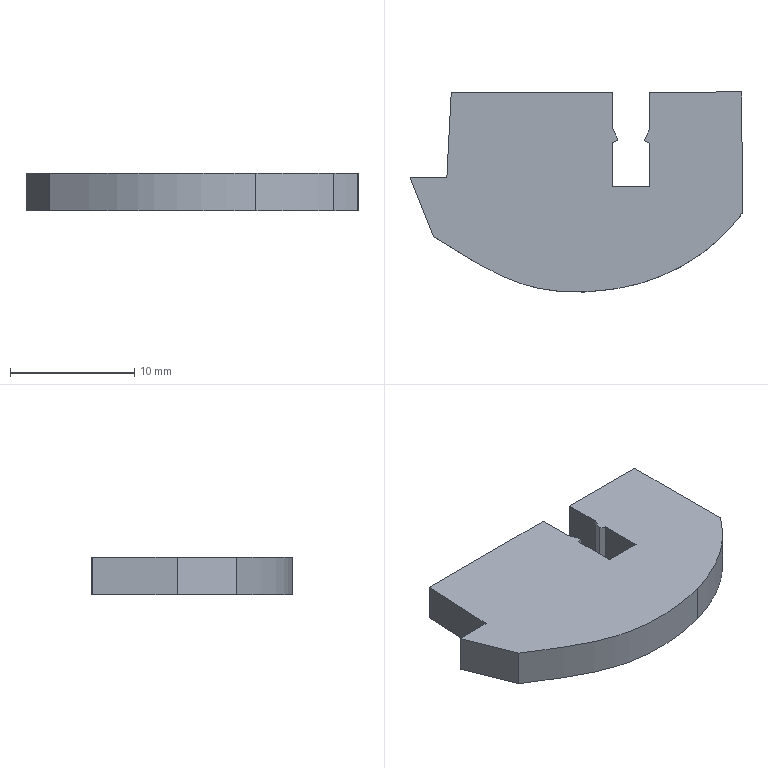Part | SolidWorks | features BaseBody 1 | 1 solid | 22 faces | box 26.677 x 16.089 x 3 mm | volume 988.858 mm3 | plane 18 | spline 4
STEP:
#1=CARTESIAN_POINT('',(-14.822,-11.074,-1.5));
#2=VERTEX_POINT('',#1);
#3=CARTESIAN_POINT('',(-16.703,-6.31,-1.5));
#4=VERTEX_POINT('',#3);
#5=CARTESIAN_POINT('',(-16.606,-6.554,-1.5));
#6=DIRECTION('',(-0.3671,0.9302,0.));
#7=VECTOR('',#6,1000.);
#8=LINE('',#5,#7);
#9=EDGE_CURVE('',#2,#4,#8,.T.);
#10=ORIENTED_EDGE('',*,*,#9,.T.);
#11=CARTESIAN_POINT('',(-13.741,-6.302,-1.5));
#12=VERTEX_POINT('',#11);
#13=CARTESIAN_POINT('',(0.01595,-6.267,-1.5));
#14=DIRECTION('',(1.,0.002545,0.));
#15=VECTOR('',#14,1000.);
#16=LINE('',#13,#15);
#17=EDGE_CURVE('',#4,#12,#16,.T.);
#18=ORIENTED_EDGE('',*,*,#17,.T.);
#19=CARTESIAN_POINT('',(-13.391,0.4792,-1.5));
#20=VERTEX_POINT('',#19);
#21=CARTESIAN_POINT('',(-13.381,0.6903,-1.5));
#22=DIRECTION('',(0.05152,0.9987,0.));
#23=VECTOR('',#22,1000.);
#24=LINE('',#21,#23);
#25=EDGE_CURVE('',#12,#20,#24,.T.);
#26=ORIENTED_EDGE('',*,*,#25,.T.);
#27=CARTESIAN_POINT('',(-0.4409,0.5122,-1.5));
#28=VERTEX_POINT('',#27);
#29=CARTESIAN_POINT('',(-0.001307,0.5133,-1.5));
#30=DIRECTION('',(1.,0.002545,0.));
#31=VECTOR('',#30,1000.);
#32=LINE('',#29,#31);
#33=EDGE_CURVE('',#20,#28,#32,.T.);
#34=ORIENTED_EDGE('',*,*,#33,.T.);
#35=CARTESIAN_POINT('',(-0.4409,-2.331,-1.5));
#36=VERTEX_POINT('',#35);
#37=CARTESIAN_POINT('',(-0.4409,0.,-1.5));
#38=DIRECTION('',(0.,1.,0.));
#39=VECTOR('',#38,1000.);
#40=LINE('',#37,#39);
#41=EDGE_CURVE('',#36,#28,#40,.T.);
#42=ORIENTED_EDGE('',*,*,#41,.F.);
#43=CARTESIAN_POINT('',(0.008047,-3.34,-1.5));
#44=VERTEX_POINT('',#43);
#45=CARTESIAN_POINT('',(-1.234,-0.5495,-1.5));
#46=DIRECTION('',(-0.4068,0.9135,0.));
#47=VECTOR('',#46,1000.);
#48=LINE('',#45,#47);
#49=EDGE_CURVE('',#44,#36,#48,.T.);
#50=ORIENTED_EDGE('',*,*,#49,.F.);
#51=CARTESIAN_POINT('',(-0.4409,-3.537,-1.5));
#52=VERTEX_POINT('',#51);
#53=CARTESIAN_POINT('',(1.232,-2.801,-1.5));
#54=DIRECTION('',(0.9154,0.4025,0.));
#55=VECTOR('',#54,1000.);
#56=LINE('',#53,#55);
#57=EDGE_CURVE('',#52,#44,#56,.T.);
#58=ORIENTED_EDGE('',*,*,#57,.F.);
#59=CARTESIAN_POINT('',(-0.4409,-7.047,-1.5));
#60=VERTEX_POINT('',#59);
#61=CARTESIAN_POINT('',(-0.4409,0.,-1.5));
#62=DIRECTION('',(0.,1.,0.));
#63=VECTOR('',#62,1000.);
#64=LINE('',#61,#63);
#65=EDGE_CURVE('',#60,#52,#64,.T.);
#66=ORIENTED_EDGE('',*,*,#65,.F.);
#67=CARTESIAN_POINT('',(2.555,-7.047,-1.5));
#68=VERTEX_POINT('',#67);
#69=CARTESIAN_POINT('',(0.,-7.047,-1.5));
#70=DIRECTION('',(-1.,0.,0.));
#71=VECTOR('',#70,1000.);
#72=LINE('',#69,#71);
#73=EDGE_CURVE('',#68,#60,#72,.T.);
#74=ORIENTED_EDGE('',*,*,#73,.F.);
#75=CARTESIAN_POINT('',(2.555,-3.572,-1.5));
#76=VERTEX_POINT('',#75);
#77=CARTESIAN_POINT('',(2.555,0.,-1.5));
#78=DIRECTION('',(0.,-1.,0.));
#79=VECTOR('',#78,1000.);
#80=LINE('',#77,#79);
#81=EDGE_CURVE('',#76,#68,#80,.T.);
#82=ORIENTED_EDGE('',*,*,#81,.F.);
#83=CARTESIAN_POINT('',(2.106,-3.373,-1.5));
#84=VERTEX_POINT('',#83);
#85=CARTESIAN_POINT('',(-0.904,-2.036,-1.5));
#86=DIRECTION('',(0.914,-0.4058,0.));
#87=VECTOR('',#86,1000.);
#88=LINE('',#85,#87);
#89=EDGE_CURVE('',#84,#76,#88,.T.);
#90=ORIENTED_EDGE('',*,*,#89,.F.);
#91=CARTESIAN_POINT('',(2.555,-2.414,-1.5));
#92=VERTEX_POINT('',#91);
#93=CARTESIAN_POINT('',(3.023,-1.416,-1.5));
#94=DIRECTION('',(-0.4242,-0.9056,0.));
#95=VECTOR('',#94,1000.);
#96=LINE('',#93,#95);
#97=EDGE_CURVE('',#92,#84,#96,.T.);
#98=ORIENTED_EDGE('',*,*,#97,.F.);
#99=CARTESIAN_POINT('',(2.555,0.5198,-1.5));
#100=VERTEX_POINT('',#99);
#101=CARTESIAN_POINT('',(2.555,0.,-1.5));
#102=DIRECTION('',(0.,-1.,0.));
#103=VECTOR('',#102,1000.);
#104=LINE('',#101,#103);
#105=EDGE_CURVE('',#100,#92,#104,.T.);
#106=ORIENTED_EDGE('',*,*,#105,.F.);
#107=CARTESIAN_POINT('',(9.963,0.5387,-1.5));
#108=VERTEX_POINT('',#107);
#109=CARTESIAN_POINT('',(-0.001307,0.5133,-1.5));
#110=DIRECTION('',(1.,0.002545,0.));
#111=VECTOR('',#110,1000.);
#112=LINE('',#109,#111);
#113=EDGE_CURVE('',#100,#108,#112,.T.);
#114=ORIENTED_EDGE('',*,*,#113,.T.);
#115=CARTESIAN_POINT('',(9.974,-3.538,-1.5));
#116=VERTEX_POINT('',#115);
#117=CARTESIAN_POINT('',(9.965,0.02536,-1.5));
#118=DIRECTION('',(0.002545,-1.,0.));
#119=VECTOR('',#118,1000.);
#120=LINE('',#117,#119);
#121=EDGE_CURVE('',#108,#116,#120,.T.);
#122=ORIENTED_EDGE('',*,*,#121,.T.);
#123=CARTESIAN_POINT('',(9.974,-9.237,-1.5));
#124=VERTEX_POINT('',#123);
#125=CARTESIAN_POINT('',(9.974,0.,-1.5));
#126=DIRECTION('',(0.,-1.,0.));
#127=VECTOR('',#126,1000.);
#128=LINE('',#125,#127);
#129=EDGE_CURVE('',#116,#124,#128,.T.);
#130=ORIENTED_EDGE('',*,*,#129,.T.);
#131=CARTESIAN_POINT('',(9.954,-9.263,-1.5));
#132=VERTEX_POINT('',#131);
#133=CARTESIAN_POINT('',(9.974,-9.237,-1.5));
#134=CARTESIAN_POINT('',(9.967,-9.246,-1.5));
#135=CARTESIAN_POINT('',(9.961,-9.255,-1.5));
#136=CARTESIAN_POINT('',(9.954,-9.263,-1.5));
#137=B_SPLINE_CURVE_WITH_KNOTS('',3,(#133,#134,#135,#136),.UNSPECIFIED.,.F.,.F.,(4,4),(0.5,0.5003),.UNSPECIFIED.);
#138=EDGE_CURVE('',#124,#132,#137,.T.);
#139=ORIENTED_EDGE('',*,*,#138,.T.);
#140=CARTESIAN_POINT('',(8.037,-11.399,-1.5));
#141=VERTEX_POINT('',#140);
#142=CARTESIAN_POINT('',(8.037,-11.399,-1.5));
#143=CARTESIAN_POINT('',(8.294,-11.148,-1.5));
#144=CARTESIAN_POINT('',(8.961,-10.455,-1.5));
#145=CARTESIAN_POINT('',(9.572,-9.722,-1.5));
#146=CARTESIAN_POINT('',(9.954,-9.263,-1.5));
#147=B_SPLINE_CURVE_WITH_KNOTS('',3,(#142,#143,#144,#145,#146),.UNSPECIFIED.,.F.,.F.,(4,1,4),(0.895,0.9336,0.9981),.UNSPECIFIED.);
#148=EDGE_CURVE('',#141,#132,#147,.T.);
#149=ORIENTED_EDGE('',*,*,#148,.F.);
#150=CARTESIAN_POINT('',(1.771,-14.856,-1.5));
#151=VERTEX_POINT('',#150);
#152=CARTESIAN_POINT('',(8.037,-11.399,-1.5));
#153=CARTESIAN_POINT('',(6.42,-12.884,-1.5));
#154=CARTESIAN_POINT('',(4.367,-14.099,-1.5));
#155=CARTESIAN_POINT('',(1.771,-14.856,-1.5));
#156=B_SPLINE_CURVE_WITH_KNOTS('',3,(#152,#153,#154,#155),.UNSPECIFIED.,.F.,.F.,(4,4),(0.5252,0.5809),.UNSPECIFIED.);
#157=EDGE_CURVE('',#141,#151,#156,.T.);
#158=ORIENTED_EDGE('',*,*,#157,.T.);
#159=CARTESIAN_POINT('',(-14.822,-11.074,-1.5));
#160=CARTESIAN_POINT('',(-13.537,-11.899,-1.5));
#161=CARTESIAN_POINT('',(-11.104,-13.46,-1.5));
#162=CARTESIAN_POINT('',(-7.073,-15.339,-1.5));
#163=CARTESIAN_POINT('',(-2.98,-15.702,-1.5));
#164=CARTESIAN_POINT('',(-0.01753,-15.28,-1.5));
#165=CARTESIAN_POINT('',(1.443,-14.941,-1.5));
#166=CARTESIAN_POINT('',(1.771,-14.856,-1.5));
#167=B_SPLINE_CURVE_WITH_KNOTS('',3,(#159,#160,#161,#162,#163,#164,#165,#166),.UNSPECIFIED.,.F.,.F.,(4,1,1,1,1,4),(0.,0.1649,0.3121,0.4748,0.5989,0.6352),.UNSPECIFIED.);
#168=EDGE_CURVE('',#2,#151,#167,.T.);
#169=ORIENTED_EDGE('',*,*,#168,.F.);
#170=EDGE_LOOP('',(#10,#18,#26,#34,#42,#50,#58,#66,#74,#82,#90,#98,#106,#114,#122,#130,#139,#149,#158,#169));
#171=FACE_OUTER_BOUND('',#170,.T.);
#172=CARTESIAN_POINT('',(0.,0.,-1.5));
#173=DIRECTION('',(0.,0.,1.));
#174=DIRECTION('',(1.,0.,0.));
#175=AXIS2_PLACEMENT_3D('',#172,#173,#174);
#176=PLANE('',#175);
#177=ADVANCED_FACE('',(#171),#176,.F.);
#178=CARTESIAN_POINT('',(-14.822,-11.074,1.5));
#179=VERTEX_POINT('',#178);
#180=CARTESIAN_POINT('',(-16.703,-6.31,1.5));
#181=VERTEX_POINT('',#180);
#182=CARTESIAN_POINT('',(-16.606,-6.554,1.5));
#183=DIRECTION('',(-0.3671,0.9302,0.));
#184=VECTOR('',#183,1000.);
#185=LINE('',#182,#184);
#186=EDGE_CURVE('',#179,#181,#185,.T.);
#187=ORIENTED_EDGE('',*,*,#186,.F.);
#188=CARTESIAN_POINT('',(1.771,-14.856,1.5));
#189=VERTEX_POINT('',#188);
#190=CARTESIAN_POINT('',(-14.822,-11.074,1.5));
#191=CARTESIAN_POINT('',(-13.537,-11.899,1.5));
#192=CARTESIAN_POINT('',(-11.104,-13.46,1.5));
#193=CARTESIAN_POINT('',(-7.073,-15.339,1.5));
#194=CARTESIAN_POINT('',(-2.98,-15.702,1.5));
#195=CARTESIAN_POINT('',(-0.01753,-15.28,1.5));
#196=CARTESIAN_POINT('',(1.443,-14.941,1.5));
#197=CARTESIAN_POINT('',(1.771,-14.856,1.5));
#198=B_SPLINE_CURVE_WITH_KNOTS('',3,(#190,#191,#192,#193,#194,#195,#196,#197),.UNSPECIFIED.,.F.,.F.,(4,1,1,1,1,4),(0.,0.1649,0.3121,0.4748,0.5989,0.6352),.UNSPECIFIED.);
#199=EDGE_CURVE('',#179,#189,#198,.T.);
#200=ORIENTED_EDGE('',*,*,#199,.T.);
#201=CARTESIAN_POINT('',(8.037,-11.399,1.5));
#202=VERTEX_POINT('',#201);
#203=CARTESIAN_POINT('',(8.037,-11.399,1.5));
#204=CARTESIAN_POINT('',(6.42,-12.884,1.5));
#205=CARTESIAN_POINT('',(4.367,-14.099,1.5));
#206=CARTESIAN_POINT('',(1.771,-14.856,1.5));
#207=B_SPLINE_CURVE_WITH_KNOTS('',3,(#203,#204,#205,#206),.UNSPECIFIED.,.F.,.F.,(4,4),(0.5252,0.5809),.UNSPECIFIED.);
#208=EDGE_CURVE('',#202,#189,#207,.T.);
#209=ORIENTED_EDGE('',*,*,#208,.F.);
#210=CARTESIAN_POINT('',(9.954,-9.263,1.5));
#211=VERTEX_POINT('',#210);
#212=CARTESIAN_POINT('',(8.037,-11.399,1.5));
#213=CARTESIAN_POINT('',(8.294,-11.148,1.5));
#214=CARTESIAN_POINT('',(8.961,-10.455,1.5));
#215=CARTESIAN_POINT('',(9.572,-9.722,1.5));
#216=CARTESIAN_POINT('',(9.954,-9.263,1.5));
#217=B_SPLINE_CURVE_WITH_KNOTS('',3,(#212,#213,#214,#215,#216),.UNSPECIFIED.,.F.,.F.,(4,1,4),(0.895,0.9336,0.9981),.UNSPECIFIED.);
#218=EDGE_CURVE('',#202,#211,#217,.T.);
#219=ORIENTED_EDGE('',*,*,#218,.T.);
#220=CARTESIAN_POINT('',(9.974,-9.237,1.5));
#221=VERTEX_POINT('',#220);
#222=CARTESIAN_POINT('',(9.974,-9.237,1.5));
#223=CARTESIAN_POINT('',(9.967,-9.246,1.5));
#224=CARTESIAN_POINT('',(9.961,-9.255,1.5));
#225=CARTESIAN_POINT('',(9.954,-9.263,1.5));
#226=B_SPLINE_CURVE_WITH_KNOTS('',3,(#222,#223,#224,#225),.UNSPECIFIED.,.F.,.F.,(4,4),(0.5,0.5003),.UNSPECIFIED.);
#227=EDGE_CURVE('',#221,#211,#226,.T.);
#228=ORIENTED_EDGE('',*,*,#227,.F.);
#229=CARTESIAN_POINT('',(9.974,-3.538,1.5));
#230=VERTEX_POINT('',#229);
#231=CARTESIAN_POINT('',(9.974,0.,1.5));
#232=DIRECTION('',(0.,-1.,0.));
#233=VECTOR('',#232,1000.);
#234=LINE('',#231,#233);
#235=EDGE_CURVE('',#230,#221,#234,.T.);
#236=ORIENTED_EDGE('',*,*,#235,.F.);
#237=CARTESIAN_POINT('',(9.963,0.5387,1.5));
#238=VERTEX_POINT('',#237);
#239=CARTESIAN_POINT('',(9.965,0.02536,1.5));
#240=DIRECTION('',(0.002545,-1.,0.));
#241=VECTOR('',#240,1000.);
#242=LINE('',#239,#241);
#243=EDGE_CURVE('',#238,#230,#242,.T.);
#244=ORIENTED_EDGE('',*,*,#243,.F.);
#245=CARTESIAN_POINT('',(2.555,0.5198,1.5));
#246=VERTEX_POINT('',#245);
#247=CARTESIAN_POINT('',(-0.001307,0.5133,1.5));
#248=DIRECTION('',(1.,0.002545,0.));
#249=VECTOR('',#248,1000.);
#250=LINE('',#247,#249);
#251=EDGE_CURVE('',#246,#238,#250,.T.);
#252=ORIENTED_EDGE('',*,*,#251,.F.);
#253=CARTESIAN_POINT('',(2.555,-2.414,1.5));
#254=VERTEX_POINT('',#253);
#255=CARTESIAN_POINT('',(2.555,0.,1.5));
#256=DIRECTION('',(0.,-1.,0.));
#257=VECTOR('',#256,1000.);
#258=LINE('',#255,#257);
#259=EDGE_CURVE('',#246,#254,#258,.T.);
#260=ORIENTED_EDGE('',*,*,#259,.T.);
#261=CARTESIAN_POINT('',(2.106,-3.373,1.5));
#262=VERTEX_POINT('',#261);
#263=CARTESIAN_POINT('',(3.023,-1.416,1.5));
#264=DIRECTION('',(-0.4242,-0.9056,0.));
#265=VECTOR('',#264,1000.);
#266=LINE('',#263,#265);
#267=EDGE_CURVE('',#254,#262,#266,.T.);
#268=ORIENTED_EDGE('',*,*,#267,.T.);
#269=CARTESIAN_POINT('',(2.555,-3.572,1.5));
#270=VERTEX_POINT('',#269);
#271=CARTESIAN_POINT('',(-0.904,-2.036,1.5));
#272=DIRECTION('',(0.914,-0.4058,0.));
#273=VECTOR('',#272,1000.);
#274=LINE('',#271,#273);
#275=EDGE_CURVE('',#262,#270,#274,.T.);
#276=ORIENTED_EDGE('',*,*,#275,.T.);
#277=CARTESIAN_POINT('',(2.555,-7.047,1.5));
#278=VERTEX_POINT('',#277);
#279=CARTESIAN_POINT('',(2.555,0.,1.5));
#280=DIRECTION('',(0.,-1.,0.));
#281=VECTOR('',#280,1000.);
#282=LINE('',#279,#281);
#283=EDGE_CURVE('',#270,#278,#282,.T.);
#284=ORIENTED_EDGE('',*,*,#283,.T.);
#285=CARTESIAN_POINT('',(-0.4409,-7.047,1.5));
#286=VERTEX_POINT('',#285);
#287=CARTESIAN_POINT('',(0.,-7.047,1.5));
#288=DIRECTION('',(-1.,0.,0.));
#289=VECTOR('',#288,1000.);
#290=LINE('',#287,#289);
#291=EDGE_CURVE('',#278,#286,#290,.T.);
#292=ORIENTED_EDGE('',*,*,#291,.T.);
#293=CARTESIAN_POINT('',(-0.4409,-3.537,1.5));
#294=VERTEX_POINT('',#293);
#295=CARTESIAN_POINT('',(-0.4409,0.,1.5));
#296=DIRECTION('',(0.,1.,0.));
#297=VECTOR('',#296,1000.);
#298=LINE('',#295,#297);
#299=EDGE_CURVE('',#286,#294,#298,.T.);
#300=ORIENTED_EDGE('',*,*,#299,.T.);
#301=CARTESIAN_POINT('',(0.008047,-3.34,1.5));
#302=VERTEX_POINT('',#301);
#303=CARTESIAN_POINT('',(1.232,-2.801,1.5));
#304=DIRECTION('',(0.9154,0.4025,0.));
#305=VECTOR('',#304,1000.);
#306=LINE('',#303,#305);
#307=EDGE_CURVE('',#294,#302,#306,.T.);
#308=ORIENTED_EDGE('',*,*,#307,.T.);
#309=CARTESIAN_POINT('',(-0.4409,-2.331,1.5));
#310=VERTEX_POINT('',#309);
#311=CARTESIAN_POINT('',(-1.234,-0.5495,1.5));
#312=DIRECTION('',(-0.4068,0.9135,0.));
#313=VECTOR('',#312,1000.);
#314=LINE('',#311,#313);
#315=EDGE_CURVE('',#302,#310,#314,.T.);
#316=ORIENTED_EDGE('',*,*,#315,.T.);
#317=CARTESIAN_POINT('',(-0.4409,0.5122,1.5));
#318=VERTEX_POINT('',#317);
#319=CARTESIAN_POINT('',(-0.4409,0.,1.5));
#320=DIRECTION('',(0.,1.,0.));
#321=VECTOR('',#320,1000.);
#322=LINE('',#319,#321);
#323=EDGE_CURVE('',#310,#318,#322,.T.);
#324=ORIENTED_EDGE('',*,*,#323,.T.);
#325=CARTESIAN_POINT('',(-13.391,0.4792,1.5));
#326=VERTEX_POINT('',#325);
#327=CARTESIAN_POINT('',(-0.001307,0.5133,1.5));
#328=DIRECTION('',(1.,0.002545,0.));
#329=VECTOR('',#328,1000.);
#330=LINE('',#327,#329);
#331=EDGE_CURVE('',#326,#318,#330,.T.);
#332=ORIENTED_EDGE('',*,*,#331,.F.);
#333=CARTESIAN_POINT('',(-13.741,-6.302,1.5));
#334=VERTEX_POINT('',#333);
#335=CARTESIAN_POINT('',(-13.381,0.6903,1.5));
#336=DIRECTION('',(0.05152,0.9987,0.));
#337=VECTOR('',#336,1000.);
#338=LINE('',#335,#337);
#339=EDGE_CURVE('',#334,#326,#338,.T.);
#340=ORIENTED_EDGE('',*,*,#339,.F.);
#341=CARTESIAN_POINT('',(0.01595,-6.267,1.5));
#342=DIRECTION('',(1.,0.002545,0.));
#343=VECTOR('',#342,1000.);
#344=LINE('',#341,#343);
#345=EDGE_CURVE('',#181,#334,#344,.T.);
#346=ORIENTED_EDGE('',*,*,#345,.F.);
#347=EDGE_LOOP('',(#187,#200,#209,#219,#228,#236,#244,#252,#260,#268,#276,#284,#292,#300,#308,#316,#324,#332,#340,#346));
#348=FACE_OUTER_BOUND('',#347,.T.);
#349=CARTESIAN_POINT('',(0.,0.,1.5));
#350=DIRECTION('',(0.,0.,1.));
#351=DIRECTION('',(1.,0.,0.));
#352=AXIS2_PLACEMENT_3D('',#349,#350,#351);
#353=PLANE('',#352);
#354=ADVANCED_FACE('',(#348),#353,.T.);
#355=ORIENTED_EDGE('',*,*,#17,.F.);
#356=CARTESIAN_POINT('',(-16.703,-6.31,1.5));
#357=DIRECTION('',(0.,0.,-1.));
#358=VECTOR('',#357,1000.);
#359=LINE('',#356,#358);
#360=EDGE_CURVE('',#181,#4,#359,.T.);
#361=ORIENTED_EDGE('',*,*,#360,.F.);
#362=ORIENTED_EDGE('',*,*,#345,.T.);
#363=CARTESIAN_POINT('',(-13.741,-6.302,1.5));
#364=DIRECTION('',(0.,0.,-1.));
#365=VECTOR('',#364,1000.);
#366=LINE('',#363,#365);
#367=EDGE_CURVE('',#334,#12,#366,.T.);
#368=ORIENTED_EDGE('',*,*,#367,.T.);
#369=EDGE_LOOP('',(#355,#361,#362,#368));
#370=FACE_OUTER_BOUND('',#369,.T.);
#371=CARTESIAN_POINT('',(0.01595,-6.267,1.5));
#372=DIRECTION('',(-0.002545,1.,0.));
#373=DIRECTION('',(0.,0.,1.));
#374=AXIS2_PLACEMENT_3D('',#371,#372,#373);
#375=PLANE('',#374);
#376=ADVANCED_FACE('',(#370),#375,.T.);
#377=ORIENTED_EDGE('',*,*,#25,.F.);
#378=ORIENTED_EDGE('',*,*,#367,.F.);
#379=ORIENTED_EDGE('',*,*,#339,.T.);
#380=CARTESIAN_POINT('',(-13.391,0.4792,1.5));
#381=DIRECTION('',(0.,0.,-1.));
#382=VECTOR('',#381,1000.);
#383=LINE('',#380,#382);
#384=EDGE_CURVE('',#326,#20,#383,.T.);
#385=ORIENTED_EDGE('',*,*,#384,.T.);
#386=EDGE_LOOP('',(#377,#378,#379,#385));
#387=FACE_OUTER_BOUND('',#386,.T.);
#388=CARTESIAN_POINT('',(-13.381,0.6903,1.5));
#389=DIRECTION('',(-0.9987,0.05152,0.));
#390=DIRECTION('',(0.,0.,1.));
#391=AXIS2_PLACEMENT_3D('',#388,#389,#390);
#392=PLANE('',#391);
#393=ADVANCED_FACE('',(#387),#392,.T.);
#394=ORIENTED_EDGE('',*,*,#33,.F.);
#395=ORIENTED_EDGE('',*,*,#384,.F.);
#396=ORIENTED_EDGE('',*,*,#331,.T.);
#397=CARTESIAN_POINT('',(-0.4409,0.5122,1.5));
#398=DIRECTION('',(0.,0.,-1.));
#399=VECTOR('',#398,1000.);
#400=LINE('',#397,#399);
#401=EDGE_CURVE('',#318,#28,#400,.T.);
#402=ORIENTED_EDGE('',*,*,#401,.T.);
#403=EDGE_LOOP('',(#394,#395,#396,#402));
#404=FACE_OUTER_BOUND('',#403,.T.);
#405=CARTESIAN_POINT('',(-0.001307,0.5133,1.5));
#406=DIRECTION('',(-0.002545,1.,0.));
#407=DIRECTION('',(0.,0.,1.));
#408=AXIS2_PLACEMENT_3D('',#405,#406,#407);
#409=PLANE('',#408);
#410=ADVANCED_FACE('',(#404),#409,.T.);
#411=ORIENTED_EDGE('',*,*,#41,.T.);
#412=ORIENTED_EDGE('',*,*,#401,.F.);
#413=ORIENTED_EDGE('',*,*,#323,.F.);
#414=CARTESIAN_POINT('',(-0.4409,-2.331,1.5));
#415=DIRECTION('',(0.,0.,-1.));
#416=VECTOR('',#415,1000.);
#417=LINE('',#414,#416);
#418=EDGE_CURVE('',#310,#36,#417,.T.);
#419=ORIENTED_EDGE('',*,*,#418,.T.);
#420=EDGE_LOOP('',(#411,#412,#413,#419));
#421=FACE_OUTER_BOUND('',#420,.T.);
#422=CARTESIAN_POINT('',(-0.4409,0.,1.5));
#423=DIRECTION('',(-1.,0.,0.));
#424=DIRECTION('',(0.,0.,1.));
#425=AXIS2_PLACEMENT_3D('',#422,#423,#424);
#426=PLANE('',#425);
#427=ADVANCED_FACE('',(#421),#426,.F.);
#428=ORIENTED_EDGE('',*,*,#49,.T.);
#429=ORIENTED_EDGE('',*,*,#418,.F.);
#430=ORIENTED_EDGE('',*,*,#315,.F.);
#431=CARTESIAN_POINT('',(0.008047,-3.34,1.5));
#432=DIRECTION('',(0.,0.,-1.));
#433=VECTOR('',#432,1000.);
#434=LINE('',#431,#433);
#435=EDGE_CURVE('',#302,#44,#434,.T.);
#436=ORIENTED_EDGE('',*,*,#435,.T.);
#437=EDGE_LOOP('',(#428,#429,#430,#436));
#438=FACE_OUTER_BOUND('',#437,.T.);
#439=CARTESIAN_POINT('',(-1.234,-0.5495,1.5));
#440=DIRECTION('',(-0.9135,-0.4068,0.));
#441=DIRECTION('',(-0.4068,0.9135,0.));
#442=AXIS2_PLACEMENT_3D('',#439,#440,#441);
#443=PLANE('',#442);
#444=ADVANCED_FACE('',(#438),#443,.F.);
#445=ORIENTED_EDGE('',*,*,#57,.T.);
#446=ORIENTED_EDGE('',*,*,#435,.F.);
#447=ORIENTED_EDGE('',*,*,#307,.F.);
#448=CARTESIAN_POINT('',(-0.4409,-3.537,1.5));
#449=DIRECTION('',(0.,0.,-1.));
#450=VECTOR('',#449,1000.);
#451=LINE('',#448,#450);
#452=EDGE_CURVE('',#294,#52,#451,.T.);
#453=ORIENTED_EDGE('',*,*,#452,.T.);
#454=EDGE_LOOP('',(#445,#446,#447,#453));
#455=FACE_OUTER_BOUND('',#454,.T.);
#456=CARTESIAN_POINT('',(1.232,-2.801,1.5));
#457=DIRECTION('',(-0.4025,0.9154,0.));
#458=DIRECTION('',(0.,0.,1.));
#459=AXIS2_PLACEMENT_3D('',#456,#457,#458);
#460=PLANE('',#459);
#461=ADVANCED_FACE('',(#455),#460,.F.);
#462=ORIENTED_EDGE('',*,*,#65,.T.);
#463=ORIENTED_EDGE('',*,*,#452,.F.);
#464=ORIENTED_EDGE('',*,*,#299,.F.);
#465=CARTESIAN_POINT('',(-0.4409,-7.047,1.5));
#466=DIRECTION('',(0.,0.,-1.));
#467=VECTOR('',#466,1000.);
#468=LINE('',#465,#467);
#469=EDGE_CURVE('',#286,#60,#468,.T.);
#470=ORIENTED_EDGE('',*,*,#469,.T.);
#471=EDGE_LOOP('',(#462,#463,#464,#470));
#472=FACE_OUTER_BOUND('',#471,.T.);
#473=CARTESIAN_POINT('',(-0.4409,0.,1.5));
#474=DIRECTION('',(-1.,0.,0.));
#475=DIRECTION('',(0.,0.,1.));
#476=AXIS2_PLACEMENT_3D('',#473,#474,#475);
#477=PLANE('',#476);
#478=ADVANCED_FACE('',(#472),#477,.F.);
#479=ORIENTED_EDGE('',*,*,#73,.T.);
#480=ORIENTED_EDGE('',*,*,#469,.F.);
#481=ORIENTED_EDGE('',*,*,#291,.F.);
#482=CARTESIAN_POINT('',(2.555,-7.047,1.5));
#483=DIRECTION('',(0.,0.,-1.));
#484=VECTOR('',#483,1000.);
#485=LINE('',#482,#484);
#486=EDGE_CURVE('',#278,#68,#485,.T.);
#487=ORIENTED_EDGE('',*,*,#486,.T.);
#488=EDGE_LOOP('',(#479,#480,#481,#487));
#489=FACE_OUTER_BOUND('',#488,.T.);
#490=CARTESIAN_POINT('',(0.,-7.047,1.5));
#491=DIRECTION('',(0.,-1.,0.));
#492=DIRECTION('',(0.,0.,-1.));
#493=AXIS2_PLACEMENT_3D('',#490,#491,#492);
#494=PLANE('',#493);
#495=ADVANCED_FACE('',(#489),#494,.F.);
#496=ORIENTED_EDGE('',*,*,#81,.T.);
#497=ORIENTED_EDGE('',*,*,#486,.F.);
#498=ORIENTED_EDGE('',*,*,#283,.F.);
#499=CARTESIAN_POINT('',(2.555,-3.572,1.5));
#500=DIRECTION('',(0.,0.,-1.));
#501=VECTOR('',#500,1000.);
#502=LINE('',#499,#501);
#503=EDGE_CURVE('',#270,#76,#502,.T.);
#504=ORIENTED_EDGE('',*,*,#503,.T.);
#505=EDGE_LOOP('',(#496,#497,#498,#504));
#506=FACE_OUTER_BOUND('',#505,.T.);
#507=CARTESIAN_POINT('',(2.555,0.,1.5));
#508=DIRECTION('',(1.,0.,0.));
#509=DIRECTION('',(0.,1.,0.));
#510=AXIS2_PLACEMENT_3D('',#507,#508,#509);
#511=PLANE('',#510);
#512=ADVANCED_FACE('',(#506),#511,.F.);
#513=ORIENTED_EDGE('',*,*,#89,.T.);
#514=ORIENTED_EDGE('',*,*,#503,.F.);
#515=ORIENTED_EDGE('',*,*,#275,.F.);
#516=CARTESIAN_POINT('',(2.106,-3.373,1.5));
#517=DIRECTION('',(0.,0.,-1.));
#518=VECTOR('',#517,1000.);
#519=LINE('',#516,#518);
#520=EDGE_CURVE('',#262,#84,#519,.T.);
#521=ORIENTED_EDGE('',*,*,#520,.T.);
#522=EDGE_LOOP('',(#513,#514,#515,#521));
#523=FACE_OUTER_BOUND('',#522,.T.);
#524=CARTESIAN_POINT('',(-0.904,-2.036,1.5));
#525=DIRECTION('',(0.4058,0.914,0.));
#526=DIRECTION('',(0.,0.,-1.));
#527=AXIS2_PLACEMENT_3D('',#524,#525,#526);
#528=PLANE('',#527);
#529=ADVANCED_FACE('',(#523),#528,.F.);
#530=ORIENTED_EDGE('',*,*,#97,.T.);
#531=ORIENTED_EDGE('',*,*,#520,.F.);
#532=ORIENTED_EDGE('',*,*,#267,.F.);
#533=CARTESIAN_POINT('',(2.555,-2.414,1.5));
#534=DIRECTION('',(0.,0.,-1.));
#535=VECTOR('',#534,1000.);
#536=LINE('',#533,#535);
#537=EDGE_CURVE('',#254,#92,#536,.T.);
#538=ORIENTED_EDGE('',*,*,#537,.T.);
#539=EDGE_LOOP('',(#530,#531,#532,#538));
#540=FACE_OUTER_BOUND('',#539,.T.);
#541=CARTESIAN_POINT('',(3.023,-1.416,1.5));
#542=DIRECTION('',(0.9056,-0.4242,0.));
#543=DIRECTION('',(0.,0.,-1.));
#544=AXIS2_PLACEMENT_3D('',#541,#542,#543);
#545=PLANE('',#544);
#546=ADVANCED_FACE('',(#540),#545,.F.);
#547=ORIENTED_EDGE('',*,*,#105,.T.);
#548=ORIENTED_EDGE('',*,*,#537,.F.);
#549=ORIENTED_EDGE('',*,*,#259,.F.);
#550=CARTESIAN_POINT('',(2.555,0.5198,1.5));
#551=DIRECTION('',(0.,0.,-1.));
#552=VECTOR('',#551,1000.);
#553=LINE('',#550,#552);
#554=EDGE_CURVE('',#246,#100,#553,.T.);
#555=ORIENTED_EDGE('',*,*,#554,.T.);
#556=EDGE_LOOP('',(#547,#548,#549,#555));
#557=FACE_OUTER_BOUND('',#556,.T.);
#558=CARTESIAN_POINT('',(2.555,0.,1.5));
#559=DIRECTION('',(1.,0.,0.));
#560=DIRECTION('',(0.,1.,0.));
#561=AXIS2_PLACEMENT_3D('',#558,#559,#560);
#562=PLANE('',#561);
#563=ADVANCED_FACE('',(#557),#562,.F.);
#564=ORIENTED_EDGE('',*,*,#113,.F.);
#565=ORIENTED_EDGE('',*,*,#554,.F.);
#566=ORIENTED_EDGE('',*,*,#251,.T.);
#567=CARTESIAN_POINT('',(9.963,0.5387,1.5));
#568=DIRECTION('',(0.,0.,-1.));
#569=VECTOR('',#568,1000.);
#570=LINE('',#567,#569);
#571=EDGE_CURVE('',#238,#108,#570,.T.);
#572=ORIENTED_EDGE('',*,*,#571,.T.);
#573=EDGE_LOOP('',(#564,#565,#566,#572));
#574=FACE_OUTER_BOUND('',#573,.T.);
#575=CARTESIAN_POINT('',(-0.001307,0.5133,1.5));
#576=DIRECTION('',(-0.002545,1.,0.));
#577=DIRECTION('',(0.,0.,1.));
#578=AXIS2_PLACEMENT_3D('',#575,#576,#577);
#579=PLANE('',#578);
#580=ADVANCED_FACE('',(#574),#579,.T.);
#581=ORIENTED_EDGE('',*,*,#121,.F.);
#582=ORIENTED_EDGE('',*,*,#571,.F.);
#583=ORIENTED_EDGE('',*,*,#243,.T.);
#584=CARTESIAN_POINT('',(9.974,-3.538,1.5));
#585=DIRECTION('',(0.,0.,-1.));
#586=VECTOR('',#585,1000.);
#587=LINE('',#584,#586);
#588=EDGE_CURVE('',#230,#116,#587,.T.);
#589=ORIENTED_EDGE('',*,*,#588,.T.);
#590=EDGE_LOOP('',(#581,#582,#583,#589));
#591=FACE_OUTER_BOUND('',#590,.T.);
#592=CARTESIAN_POINT('',(9.965,0.02536,1.5));
#593=DIRECTION('',(1.,0.002545,0.));
#594=DIRECTION('',(0.,0.,-1.));
#595=AXIS2_PLACEMENT_3D('',#592,#593,#594);
#596=PLANE('',#595);
#597=ADVANCED_FACE('',(#591),#596,.T.);
#598=ORIENTED_EDGE('',*,*,#129,.F.);
#599=ORIENTED_EDGE('',*,*,#588,.F.);
#600=ORIENTED_EDGE('',*,*,#235,.T.);
#601=CARTESIAN_POINT('',(9.974,-9.237,1.5));
#602=DIRECTION('',(0.,0.,-1.));
#603=VECTOR('',#602,1000.);
#604=LINE('',#601,#603);
#605=EDGE_CURVE('',#221,#124,#604,.T.);
#606=ORIENTED_EDGE('',*,*,#605,.T.);
#607=EDGE_LOOP('',(#598,#599,#600,#606));
#608=FACE_OUTER_BOUND('',#607,.T.);
#609=CARTESIAN_POINT('',(9.974,0.,1.5));
#610=DIRECTION('',(1.,0.,0.));
#611=DIRECTION('',(0.,1.,0.));
#612=AXIS2_PLACEMENT_3D('',#609,#610,#611);
#613=PLANE('',#612);
#614=ADVANCED_FACE('',(#608),#613,.T.);
#615=ORIENTED_EDGE('',*,*,#138,.F.);
#616=ORIENTED_EDGE('',*,*,#605,.F.);
#617=ORIENTED_EDGE('',*,*,#227,.T.);
#618=CARTESIAN_POINT('',(9.954,-9.263,1.5));
#619=DIRECTION('',(0.,0.,-1.));
#620=VECTOR('',#619,1000.);
#621=LINE('',#618,#620);
#622=EDGE_CURVE('',#211,#132,#621,.T.);
#623=ORIENTED_EDGE('',*,*,#622,.T.);
#624=EDGE_LOOP('',(#615,#616,#617,#623));
#625=FACE_OUTER_BOUND('',#624,.T.);
#626=CARTESIAN_POINT('',(9.974,-9.237,1.5));
#627=CARTESIAN_POINT('',(9.974,-9.237,-1.5));
#628=CARTESIAN_POINT('',(9.967,-9.246,1.5));
#629=CARTESIAN_POINT('',(9.967,-9.246,-1.5));
#630=CARTESIAN_POINT('',(9.961,-9.255,1.5));
#631=CARTESIAN_POINT('',(9.961,-9.255,-1.5));
#632=CARTESIAN_POINT('',(9.954,-9.263,1.5));
#633=CARTESIAN_POINT('',(9.954,-9.263,-1.5));
#634=B_SPLINE_SURFACE_WITH_KNOTS('',3,1,((#626,#627),(#628,#629),(#630,#631),(#632,#633)),.UNSPECIFIED.,.F.,.F.,.F.,(4,4),(2,2),(0.5,0.5003),(0.,1.),.UNSPECIFIED.);
#635=ADVANCED_FACE('',(#625),#634,.T.);
#636=ORIENTED_EDGE('',*,*,#148,.T.);
#637=ORIENTED_EDGE('',*,*,#622,.F.);
#638=ORIENTED_EDGE('',*,*,#218,.F.);
#639=CARTESIAN_POINT('',(8.037,-11.399,1.5));
#640=DIRECTION('',(0.,0.,-1.));
#641=VECTOR('',#640,1000.);
#642=LINE('',#639,#641);
#643=EDGE_CURVE('',#202,#141,#642,.T.);
#644=ORIENTED_EDGE('',*,*,#643,.T.);
#645=EDGE_LOOP('',(#636,#637,#638,#644));
#646=FACE_OUTER_BOUND('',#645,.T.);
#647=CARTESIAN_POINT('',(8.037,-11.399,1.5));
#648=CARTESIAN_POINT('',(8.037,-11.399,-1.5));
#649=CARTESIAN_POINT('',(8.294,-11.148,1.5));
#650=CARTESIAN_POINT('',(8.294,-11.148,-1.5));
#651=CARTESIAN_POINT('',(8.961,-10.455,1.5));
#652=CARTESIAN_POINT('',(8.961,-10.455,-1.5));
#653=CARTESIAN_POINT('',(9.572,-9.722,1.5));
#654=CARTESIAN_POINT('',(9.572,-9.722,-1.5));
#655=CARTESIAN_POINT('',(9.954,-9.263,1.5));
#656=CARTESIAN_POINT('',(9.954,-9.263,-1.5));
#657=B_SPLINE_SURFACE_WITH_KNOTS('',3,1,((#647,#648),(#649,#650),(#651,#652),(#653,#654),(#655,#656)),.UNSPECIFIED.,.F.,.F.,.F.,(4,1,4),(2,2),(0.895,0.9336,0.9981),(0.,1.),.UNSPECIFIED.);
#658=ADVANCED_FACE('',(#646),#657,.F.);
#659=ORIENTED_EDGE('',*,*,#157,.F.);
#660=ORIENTED_EDGE('',*,*,#643,.F.);
#661=ORIENTED_EDGE('',*,*,#208,.T.);
#662=CARTESIAN_POINT('',(1.771,-14.856,1.5));
#663=DIRECTION('',(0.,0.,-1.));
#664=VECTOR('',#663,1000.);
#665=LINE('',#662,#664);
#666=EDGE_CURVE('',#189,#151,#665,.T.);
#667=ORIENTED_EDGE('',*,*,#666,.T.);
#668=EDGE_LOOP('',(#659,#660,#661,#667));
#669=FACE_OUTER_BOUND('',#668,.T.);
#670=CARTESIAN_POINT('',(8.037,-11.399,1.5));
#671=CARTESIAN_POINT('',(8.037,-11.399,-1.5));
#672=CARTESIAN_POINT('',(6.42,-12.884,1.5));
#673=CARTESIAN_POINT('',(6.42,-12.884,-1.5));
#674=CARTESIAN_POINT('',(4.367,-14.099,1.5));
#675=CARTESIAN_POINT('',(4.367,-14.099,-1.5));
#676=CARTESIAN_POINT('',(1.771,-14.856,1.5));
#677=CARTESIAN_POINT('',(1.771,-14.856,-1.5));
#678=B_SPLINE_SURFACE_WITH_KNOTS('',3,1,((#670,#671),(#672,#673),(#674,#675),(#676,#677)),.UNSPECIFIED.,.F.,.F.,.F.,(4,4),(2,2),(0.5252,0.5809),(0.,1.),.UNSPECIFIED.);
#679=ADVANCED_FACE('',(#669),#678,.T.);
#680=ORIENTED_EDGE('',*,*,#168,.T.);
#681=ORIENTED_EDGE('',*,*,#666,.F.);
#682=ORIENTED_EDGE('',*,*,#199,.F.);
#683=CARTESIAN_POINT('',(-14.822,-11.074,1.5));
#684=DIRECTION('',(0.,0.,-1.));
#685=VECTOR('',#684,1000.);
#686=LINE('',#683,#685);
#687=EDGE_CURVE('',#179,#2,#686,.T.);
#688=ORIENTED_EDGE('',*,*,#687,.T.);
#689=EDGE_LOOP('',(#680,#681,#682,#688));
#690=FACE_OUTER_BOUND('',#689,.T.);
#691=CARTESIAN_POINT('',(-14.822,-11.074,1.5));
#692=CARTESIAN_POINT('',(-14.822,-11.074,-1.5));
#693=CARTESIAN_POINT('',(-13.537,-11.899,1.5));
#694=CARTESIAN_POINT('',(-13.537,-11.899,-1.5));
#695=CARTESIAN_POINT('',(-11.104,-13.46,1.5));
#696=CARTESIAN_POINT('',(-11.104,-13.46,-1.5));
#697=CARTESIAN_POINT('',(-7.073,-15.339,1.5));
#698=CARTESIAN_POINT('',(-7.073,-15.339,-1.5));
#699=CARTESIAN_POINT('',(-2.98,-15.702,1.5));
#700=CARTESIAN_POINT('',(-2.98,-15.702,-1.5));
#701=CARTESIAN_POINT('',(-0.01753,-15.28,1.5));
#702=CARTESIAN_POINT('',(-0.01753,-15.28,-1.5));
#703=CARTESIAN_POINT('',(1.443,-14.941,1.5));
#704=CARTESIAN_POINT('',(1.443,-14.941,-1.5));
#705=CARTESIAN_POINT('',(1.771,-14.856,1.5));
#706=CARTESIAN_POINT('',(1.771,-14.856,-1.5));
#707=B_SPLINE_SURFACE_WITH_KNOTS('',3,1,((#691,#692),(#693,#694),(#695,#696),(#697,#698),(#699,#700),(#701,#702),(#703,#704),(#705,#706)),.UNSPECIFIED.,.F.,.F.,.F.,(4,1,1,1,1,4),(2,2),(0.,0.1649,0.3121,0.4748,0.5989,0.6352),(0.,1.),.UNSPECIFIED.);
#708=ADVANCED_FACE('',(#690),#707,.F.);
#709=ORIENTED_EDGE('',*,*,#9,.F.);
#710=ORIENTED_EDGE('',*,*,#687,.F.);
#711=ORIENTED_EDGE('',*,*,#186,.T.);
#712=ORIENTED_EDGE('',*,*,#360,.T.);
#713=EDGE_LOOP('',(#709,#710,#711,#712));
#714=FACE_OUTER_BOUND('',#713,.T.);
#715=CARTESIAN_POINT('',(-16.606,-6.554,1.5));
#716=DIRECTION('',(-0.9302,-0.3671,0.));
#717=DIRECTION('',(-0.3671,0.9302,0.));
#718=AXIS2_PLACEMENT_3D('',#715,#716,#717);
#719=PLANE('',#718);
#720=ADVANCED_FACE('',(#714),#719,.T.);
#721=CLOSED_SHELL('',(#177,#354,#376,#393,#410,#427,#444,#461,#478,#495,#512,#529,#546,#563,#580,#597,#614,#635,#658,#679,#708,#720));
#722=MANIFOLD_SOLID_BREP('',#721);
#723=CARTESIAN_POINT('',(0.,0.,0.));
#724=DIRECTION('',(0.,0.,1.));
#725=DIRECTION('',(1.,0.,0.));
#726=AXIS2_PLACEMENT_3D('',#723,#724,#725);
#727=(LENGTH_UNIT()NAMED_UNIT(*)SI_UNIT(.MILLI.,.METRE.));
#728=UNCERTAINTY_MEASURE_WITH_UNIT(LENGTH_MEASURE(0.00001),#727,'','');
#729=(NAMED_UNIT(*)PLANE_ANGLE_UNIT()SI_UNIT($,.RADIAN.));
#730=(NAMED_UNIT(*)SI_UNIT($,.STERADIAN.)SOLID_ANGLE_UNIT());
#731=(GEOMETRIC_REPRESENTATION_CONTEXT(3)GLOBAL_UNCERTAINTY_ASSIGNED_CONTEXT((#728))GLOBAL_UNIT_ASSIGNED_CONTEXT((#727,#729,#730))REPRESENTATION_CONTEXT('',''));
#732=ADVANCED_BREP_SHAPE_REPRESENTATION('',(#722,#726),#731);